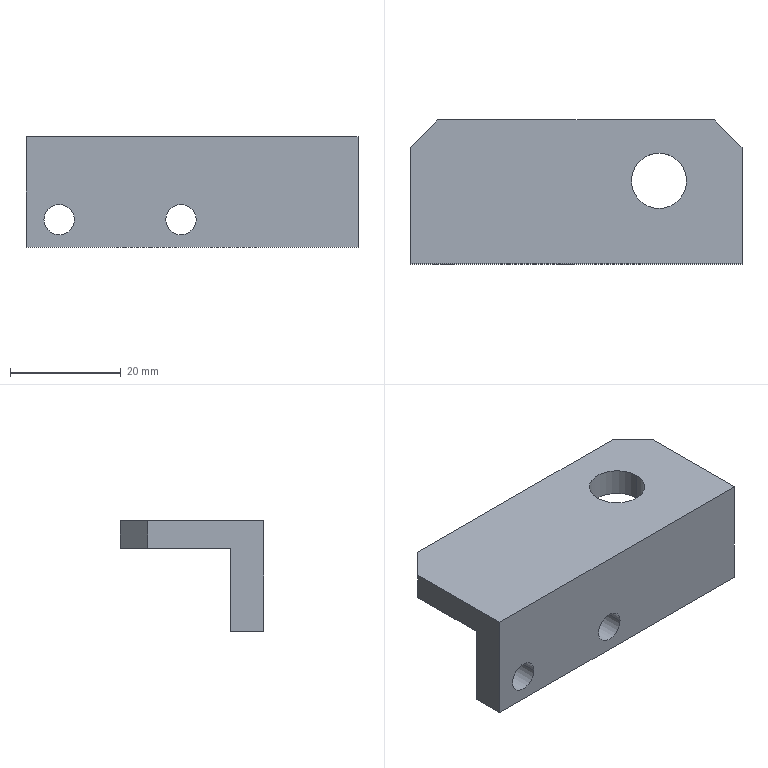Part | STEP file | push slingshot cylinder seat 2 | 1 solid | 16 faces | box 60 x 26 x 20 mm | volume 12397 mm3 | plane 10 | cylinder 6 | commonest cylinder face diameters 5.5 x4 10 x2
STEP:
#1=CARTESIAN_POINT('',(0.,0.,0.));
#2=DIRECTION('',(0.,0.,1.));
#3=DIRECTION('',(1.,0.,0.));
#4=AXIS2_PLACEMENT_3D('',#1,#2,#3);
#5=CARTESIAN_POINT('',(-9.945,-51.173,5.));
#6=VERTEX_POINT('',#5);
#7=CARTESIAN_POINT('',(-9.945,-45.173,5.));
#8=VERTEX_POINT('',#7);
#9=CARTESIAN_POINT('',(-9.945,-55.173,5.));
#10=DIRECTION('',(0.,1.,0.));
#11=VECTOR('',#10,1.);
#12=LINE('',#9,#11);
#13=CARTESIAN_POINT('',(-7.195,-55.173,5.));
#14=DIRECTION('',(0.,1.,0.));
#15=DIRECTION('',(-1.,0.,0.));
#16=AXIS2_PLACEMENT_3D('',#13,#14,#15);
#17=CYLINDRICAL_SURFACE('',#16,2.75);
#18=CARTESIAN_POINT('',(6.283,0.));
#19=DIRECTION('',(0.,1.));
#20=VECTOR('',#19,1.);
#21=LINE('',#18,#20);
#22=(GEOMETRIC_REPRESENTATION_CONTEXT(2)PARAMETRIC_REPRESENTATION_CONTEXT()REPRESENTATION_CONTEXT('',''));
#23=DEFINITIONAL_REPRESENTATION('',(#21),#22);
#24=PCURVE('',#17,#23);
#25=CARTESIAN_POINT('',(-7.195,-55.173,5.));
#26=DIRECTION('',(0.,1.,0.));
#27=DIRECTION('',(-1.,0.,0.));
#28=AXIS2_PLACEMENT_3D('',#25,#26,#27);
#29=CYLINDRICAL_SURFACE('',#28,2.75);
#30=CARTESIAN_POINT('',(0.,0.));
#31=DIRECTION('',(0.,1.));
#32=VECTOR('',#31,1.);
#33=LINE('',#30,#32);
#34=(GEOMETRIC_REPRESENTATION_CONTEXT(2)PARAMETRIC_REPRESENTATION_CONTEXT()REPRESENTATION_CONTEXT('',''));
#35=DEFINITIONAL_REPRESENTATION('',(#33),#34);
#36=PCURVE('',#29,#35);
#37=SURFACE_CURVE('',#12,(#24,#36),.PCURVE_S1.);
#38=EDGE_CURVE('',#6,#8,#37,.T.);
#39=ORIENTED_EDGE('',*,*,#38,.T.);
#40=CARTESIAN_POINT('',(-4.445,-45.173,5.));
#41=VERTEX_POINT('',#40);
#42=CARTESIAN_POINT('',(-7.195,-45.173,5.));
#43=DIRECTION('',(0.,1.,0.));
#44=DIRECTION('',(1.,0.,0.));
#45=AXIS2_PLACEMENT_3D('',#42,#43,#44);
#46=CIRCLE('',#45,2.75);
#47=CARTESIAN_POINT('',(3.142,10.));
#48=DIRECTION('',(1.,0.));
#49=VECTOR('',#48,1.);
#50=LINE('',#47,#49);
#51=(GEOMETRIC_REPRESENTATION_CONTEXT(2)PARAMETRIC_REPRESENTATION_CONTEXT()REPRESENTATION_CONTEXT('',''));
#52=DEFINITIONAL_REPRESENTATION('',(#50),#51);
#53=PCURVE('',#17,#52);
#54=CARTESIAN_POINT('',(-41.653,-45.173,-0.5459));
#55=DIRECTION('',(0.,1.,0.));
#56=DIRECTION('',(-1.,0.,0.));
#57=AXIS2_PLACEMENT_3D('',#54,#55,#56);
#58=PLANE('',#57);
#59=CARTESIAN_POINT('',(-34.458,5.546));
#60=DIRECTION('',(-1.,0.));
#61=AXIS2_PLACEMENT_2D('',#59,#60);
#62=CIRCLE('',#61,2.75);
#63=(GEOMETRIC_REPRESENTATION_CONTEXT(2)PARAMETRIC_REPRESENTATION_CONTEXT()REPRESENTATION_CONTEXT('',''));
#64=DEFINITIONAL_REPRESENTATION('',(#62),#63);
#65=PCURVE('',#58,#64);
#66=SURFACE_CURVE('',#46,(#53,#65),.PCURVE_S1.);
#67=EDGE_CURVE('',#41,#8,#66,.T.);
#68=ORIENTED_EDGE('',*,*,#67,.F.);
#69=CARTESIAN_POINT('',(-4.445,-51.173,5.));
#70=VERTEX_POINT('',#69);
#71=CARTESIAN_POINT('',(-4.445,-55.173,5.));
#72=DIRECTION('',(0.,1.,0.));
#73=VECTOR('',#72,1.);
#74=LINE('',#71,#73);
#75=CARTESIAN_POINT('',(3.142,0.));
#76=DIRECTION('',(0.,1.));
#77=VECTOR('',#76,1.);
#78=LINE('',#75,#77);
#79=(GEOMETRIC_REPRESENTATION_CONTEXT(2)PARAMETRIC_REPRESENTATION_CONTEXT()REPRESENTATION_CONTEXT('',''));
#80=DEFINITIONAL_REPRESENTATION('',(#78),#79);
#81=PCURVE('',#17,#80);
#82=CARTESIAN_POINT('',(3.142,0.));
#83=DIRECTION('',(0.,1.));
#84=VECTOR('',#83,1.);
#85=LINE('',#82,#84);
#86=(GEOMETRIC_REPRESENTATION_CONTEXT(2)PARAMETRIC_REPRESENTATION_CONTEXT()REPRESENTATION_CONTEXT('',''));
#87=DEFINITIONAL_REPRESENTATION('',(#85),#86);
#88=PCURVE('',#29,#87);
#89=SURFACE_CURVE('',#74,(#81,#88),.PCURVE_S1.);
#90=EDGE_CURVE('',#70,#41,#89,.T.);
#91=ORIENTED_EDGE('',*,*,#90,.F.);
#92=CARTESIAN_POINT('',(-7.195,-51.173,5.));
#93=DIRECTION('',(0.,1.,0.));
#94=DIRECTION('',(-1.,0.,0.));
#95=AXIS2_PLACEMENT_3D('',#92,#93,#94);
#96=CIRCLE('',#95,2.75);
#97=CARTESIAN_POINT('',(0.,4.));
#98=DIRECTION('',(1.,0.));
#99=VECTOR('',#98,1.);
#100=LINE('',#97,#99);
#101=(GEOMETRIC_REPRESENTATION_CONTEXT(2)PARAMETRIC_REPRESENTATION_CONTEXT()REPRESENTATION_CONTEXT('',''));
#102=DEFINITIONAL_REPRESENTATION('',(#100),#101);
#103=PCURVE('',#17,#102);
#104=CARTESIAN_POINT('',(-35.195,-51.173,20.));
#105=DIRECTION('',(0.,1.,0.));
#106=DIRECTION('',(-1.,0.,0.));
#107=AXIS2_PLACEMENT_3D('',#104,#105,#106);
#108=PLANE('',#107);
#109=CARTESIAN_POINT('',(-28.,-15.));
#110=DIRECTION('',(1.,0.));
#111=AXIS2_PLACEMENT_2D('',#109,#110);
#112=CIRCLE('',#111,2.75);
#113=(GEOMETRIC_REPRESENTATION_CONTEXT(2)PARAMETRIC_REPRESENTATION_CONTEXT()REPRESENTATION_CONTEXT('',''));
#114=DEFINITIONAL_REPRESENTATION('',(#112),#113);
#115=PCURVE('',#108,#114);
#116=SURFACE_CURVE('',#96,(#103,#115),.PCURVE_S1.);
#117=EDGE_CURVE('',#70,#6,#116,.T.);
#118=ORIENTED_EDGE('',*,*,#117,.T.);
#119=EDGE_LOOP('',(#39,#68,#91,#118));
#120=FACE_BOUND('',#119,.F.);
#121=ADVANCED_FACE('',(#120),#17,.F.);
#122=CARTESIAN_POINT('',(-31.945,-51.173,5.));
#123=VERTEX_POINT('',#122);
#124=CARTESIAN_POINT('',(-31.945,-45.173,5.));
#125=VERTEX_POINT('',#124);
#126=CARTESIAN_POINT('',(-31.945,-55.173,5.));
#127=DIRECTION('',(0.,1.,0.));
#128=VECTOR('',#127,1.);
#129=LINE('',#126,#128);
#130=CARTESIAN_POINT('',(-29.195,-55.173,5.));
#131=DIRECTION('',(0.,1.,0.));
#132=DIRECTION('',(-1.,0.,0.));
#133=AXIS2_PLACEMENT_3D('',#130,#131,#132);
#134=CYLINDRICAL_SURFACE('',#133,2.75);
#135=CARTESIAN_POINT('',(6.283,0.));
#136=DIRECTION('',(0.,1.));
#137=VECTOR('',#136,1.);
#138=LINE('',#135,#137);
#139=(GEOMETRIC_REPRESENTATION_CONTEXT(2)PARAMETRIC_REPRESENTATION_CONTEXT()REPRESENTATION_CONTEXT('',''));
#140=DEFINITIONAL_REPRESENTATION('',(#138),#139);
#141=PCURVE('',#134,#140);
#142=CARTESIAN_POINT('',(-29.195,-55.173,5.));
#143=DIRECTION('',(0.,1.,0.));
#144=DIRECTION('',(-1.,0.,0.));
#145=AXIS2_PLACEMENT_3D('',#142,#143,#144);
#146=CYLINDRICAL_SURFACE('',#145,2.75);
#147=CARTESIAN_POINT('',(0.,0.));
#148=DIRECTION('',(0.,1.));
#149=VECTOR('',#148,1.);
#150=LINE('',#147,#149);
#151=(GEOMETRIC_REPRESENTATION_CONTEXT(2)PARAMETRIC_REPRESENTATION_CONTEXT()REPRESENTATION_CONTEXT('',''));
#152=DEFINITIONAL_REPRESENTATION('',(#150),#151);
#153=PCURVE('',#146,#152);
#154=SURFACE_CURVE('',#129,(#141,#153),.PCURVE_S1.);
#155=EDGE_CURVE('',#123,#125,#154,.T.);
#156=ORIENTED_EDGE('',*,*,#155,.T.);
#157=CARTESIAN_POINT('',(-26.445,-45.173,5.));
#158=VERTEX_POINT('',#157);
#159=CARTESIAN_POINT('',(-29.195,-45.173,5.));
#160=DIRECTION('',(0.,1.,0.));
#161=DIRECTION('',(1.,0.,0.));
#162=AXIS2_PLACEMENT_3D('',#159,#160,#161);
#163=CIRCLE('',#162,2.75);
#164=CARTESIAN_POINT('',(3.142,10.));
#165=DIRECTION('',(1.,0.));
#166=VECTOR('',#165,1.);
#167=LINE('',#164,#166);
#168=(GEOMETRIC_REPRESENTATION_CONTEXT(2)PARAMETRIC_REPRESENTATION_CONTEXT()REPRESENTATION_CONTEXT('',''));
#169=DEFINITIONAL_REPRESENTATION('',(#167),#168);
#170=PCURVE('',#134,#169);
#171=CARTESIAN_POINT('',(-12.458,5.546));
#172=DIRECTION('',(-1.,0.));
#173=AXIS2_PLACEMENT_2D('',#171,#172);
#174=CIRCLE('',#173,2.75);
#175=(GEOMETRIC_REPRESENTATION_CONTEXT(2)PARAMETRIC_REPRESENTATION_CONTEXT()REPRESENTATION_CONTEXT('',''));
#176=DEFINITIONAL_REPRESENTATION('',(#174),#175);
#177=PCURVE('',#58,#176);
#178=SURFACE_CURVE('',#163,(#170,#177),.PCURVE_S1.);
#179=EDGE_CURVE('',#158,#125,#178,.T.);
#180=ORIENTED_EDGE('',*,*,#179,.F.);
#181=CARTESIAN_POINT('',(-26.445,-51.173,5.));
#182=VERTEX_POINT('',#181);
#183=CARTESIAN_POINT('',(-26.445,-55.173,5.));
#184=DIRECTION('',(0.,1.,0.));
#185=VECTOR('',#184,1.);
#186=LINE('',#183,#185);
#187=CARTESIAN_POINT('',(3.142,0.));
#188=DIRECTION('',(0.,1.));
#189=VECTOR('',#188,1.);
#190=LINE('',#187,#189);
#191=(GEOMETRIC_REPRESENTATION_CONTEXT(2)PARAMETRIC_REPRESENTATION_CONTEXT()REPRESENTATION_CONTEXT('',''));
#192=DEFINITIONAL_REPRESENTATION('',(#190),#191);
#193=PCURVE('',#134,#192);
#194=CARTESIAN_POINT('',(3.142,0.));
#195=DIRECTION('',(0.,1.));
#196=VECTOR('',#195,1.);
#197=LINE('',#194,#196);
#198=(GEOMETRIC_REPRESENTATION_CONTEXT(2)PARAMETRIC_REPRESENTATION_CONTEXT()REPRESENTATION_CONTEXT('',''));
#199=DEFINITIONAL_REPRESENTATION('',(#197),#198);
#200=PCURVE('',#146,#199);
#201=SURFACE_CURVE('',#186,(#193,#200),.PCURVE_S1.);
#202=EDGE_CURVE('',#182,#158,#201,.T.);
#203=ORIENTED_EDGE('',*,*,#202,.F.);
#204=CARTESIAN_POINT('',(-29.195,-51.173,5.));
#205=DIRECTION('',(0.,1.,0.));
#206=DIRECTION('',(-1.,0.,0.));
#207=AXIS2_PLACEMENT_3D('',#204,#205,#206);
#208=CIRCLE('',#207,2.75);
#209=CARTESIAN_POINT('',(0.,4.));
#210=DIRECTION('',(1.,0.));
#211=VECTOR('',#210,1.);
#212=LINE('',#209,#211);
#213=(GEOMETRIC_REPRESENTATION_CONTEXT(2)PARAMETRIC_REPRESENTATION_CONTEXT()REPRESENTATION_CONTEXT('',''));
#214=DEFINITIONAL_REPRESENTATION('',(#212),#213);
#215=PCURVE('',#134,#214);
#216=CARTESIAN_POINT('',(-6.,-15.));
#217=DIRECTION('',(1.,0.));
#218=AXIS2_PLACEMENT_2D('',#216,#217);
#219=CIRCLE('',#218,2.75);
#220=(GEOMETRIC_REPRESENTATION_CONTEXT(2)PARAMETRIC_REPRESENTATION_CONTEXT()REPRESENTATION_CONTEXT('',''));
#221=DEFINITIONAL_REPRESENTATION('',(#219),#220);
#222=PCURVE('',#108,#221);
#223=SURFACE_CURVE('',#208,(#215,#222),.PCURVE_S1.);
#224=EDGE_CURVE('',#182,#123,#223,.T.);
#225=ORIENTED_EDGE('',*,*,#224,.T.);
#226=EDGE_LOOP('',(#156,#180,#203,#225));
#227=FACE_BOUND('',#226,.F.);
#228=ADVANCED_FACE('',(#227),#134,.F.);
#229=CARTESIAN_POINT('',(4.805,-36.173,20.));
#230=VERTEX_POINT('',#229);
#231=CARTESIAN_POINT('',(4.805,-36.173,15.));
#232=VERTEX_POINT('',#231);
#233=CARTESIAN_POINT('',(4.805,-36.173,20.));
#234=DIRECTION('',(0.,0.,-1.));
#235=VECTOR('',#234,1.);
#236=LINE('',#233,#235);
#237=CARTESIAN_POINT('',(9.805,-36.173,20.));
#238=DIRECTION('',(0.,0.,-1.));
#239=DIRECTION('',(-1.,0.,0.));
#240=AXIS2_PLACEMENT_3D('',#237,#238,#239);
#241=CYLINDRICAL_SURFACE('',#240,5.);
#242=CARTESIAN_POINT('',(6.283,0.));
#243=DIRECTION('',(0.,1.));
#244=VECTOR('',#243,1.);
#245=LINE('',#242,#244);
#246=(GEOMETRIC_REPRESENTATION_CONTEXT(2)PARAMETRIC_REPRESENTATION_CONTEXT()REPRESENTATION_CONTEXT('',''));
#247=DEFINITIONAL_REPRESENTATION('',(#245),#246);
#248=PCURVE('',#241,#247);
#249=CARTESIAN_POINT('',(9.805,-36.173,20.));
#250=DIRECTION('',(0.,0.,-1.));
#251=DIRECTION('',(-1.,0.,0.));
#252=AXIS2_PLACEMENT_3D('',#249,#250,#251);
#253=CYLINDRICAL_SURFACE('',#252,5.);
#254=CARTESIAN_POINT('',(0.,0.));
#255=DIRECTION('',(0.,1.));
#256=VECTOR('',#255,1.);
#257=LINE('',#254,#256);
#258=(GEOMETRIC_REPRESENTATION_CONTEXT(2)PARAMETRIC_REPRESENTATION_CONTEXT()REPRESENTATION_CONTEXT('',''));
#259=DEFINITIONAL_REPRESENTATION('',(#257),#258);
#260=PCURVE('',#253,#259);
#261=SURFACE_CURVE('',#236,(#248,#260),.PCURVE_S1.);
#262=EDGE_CURVE('',#230,#232,#261,.T.);
#263=ORIENTED_EDGE('',*,*,#262,.T.);
#264=CARTESIAN_POINT('',(14.805,-36.173,15.));
#265=VERTEX_POINT('',#264);
#266=CARTESIAN_POINT('',(9.805,-36.173,15.));
#267=DIRECTION('',(0.,0.,1.));
#268=DIRECTION('',(1.,0.,0.));
#269=AXIS2_PLACEMENT_3D('',#266,#267,#268);
#270=CIRCLE('',#269,5.);
#271=CARTESIAN_POINT('',(9.425,5.));
#272=DIRECTION('',(-1.,0.));
#273=VECTOR('',#272,1.);
#274=LINE('',#271,#273);
#275=(GEOMETRIC_REPRESENTATION_CONTEXT(2)PARAMETRIC_REPRESENTATION_CONTEXT()REPRESENTATION_CONTEXT('',''));
#276=DEFINITIONAL_REPRESENTATION('',(#274),#275);
#277=PCURVE('',#241,#276);
#278=CARTESIAN_POINT('',(-41.653,-45.173,15.));
#279=DIRECTION('',(0.,0.,1.));
#280=DIRECTION('',(1.,0.,0.));
#281=AXIS2_PLACEMENT_3D('',#278,#279,#280);
#282=PLANE('',#281);
#283=CARTESIAN_POINT('',(51.458,9.));
#284=DIRECTION('',(1.,0.));
#285=AXIS2_PLACEMENT_2D('',#283,#284);
#286=CIRCLE('',#285,5.);
#287=(GEOMETRIC_REPRESENTATION_CONTEXT(2)PARAMETRIC_REPRESENTATION_CONTEXT()REPRESENTATION_CONTEXT('',''));
#288=DEFINITIONAL_REPRESENTATION('',(#286),#287);
#289=PCURVE('',#282,#288);
#290=SURFACE_CURVE('',#270,(#277,#289),.PCURVE_S1.);
#291=EDGE_CURVE('',#232,#265,#290,.T.);
#292=ORIENTED_EDGE('',*,*,#291,.T.);
#293=CARTESIAN_POINT('',(14.805,-36.173,20.));
#294=VERTEX_POINT('',#293);
#295=CARTESIAN_POINT('',(14.805,-36.173,20.));
#296=DIRECTION('',(0.,0.,-1.));
#297=VECTOR('',#296,1.);
#298=LINE('',#295,#297);
#299=CARTESIAN_POINT('',(3.142,0.));
#300=DIRECTION('',(0.,1.));
#301=VECTOR('',#300,1.);
#302=LINE('',#299,#301);
#303=(GEOMETRIC_REPRESENTATION_CONTEXT(2)PARAMETRIC_REPRESENTATION_CONTEXT()REPRESENTATION_CONTEXT('',''));
#304=DEFINITIONAL_REPRESENTATION('',(#302),#303);
#305=PCURVE('',#241,#304);
#306=CARTESIAN_POINT('',(3.142,0.));
#307=DIRECTION('',(0.,1.));
#308=VECTOR('',#307,1.);
#309=LINE('',#306,#308);
#310=(GEOMETRIC_REPRESENTATION_CONTEXT(2)PARAMETRIC_REPRESENTATION_CONTEXT()REPRESENTATION_CONTEXT('',''));
#311=DEFINITIONAL_REPRESENTATION('',(#309),#310);
#312=PCURVE('',#253,#311);
#313=SURFACE_CURVE('',#298,(#305,#312),.PCURVE_S1.);
#314=EDGE_CURVE('',#294,#265,#313,.T.);
#315=ORIENTED_EDGE('',*,*,#314,.F.);
#316=CARTESIAN_POINT('',(9.805,-36.173,20.));
#317=DIRECTION('',(0.,0.,1.));
#318=DIRECTION('',(1.,0.,0.));
#319=AXIS2_PLACEMENT_3D('',#316,#317,#318);
#320=CIRCLE('',#319,5.);
#321=CARTESIAN_POINT('',(9.425,0.));
#322=DIRECTION('',(-1.,0.));
#323=VECTOR('',#322,1.);
#324=LINE('',#321,#323);
#325=(GEOMETRIC_REPRESENTATION_CONTEXT(2)PARAMETRIC_REPRESENTATION_CONTEXT()REPRESENTATION_CONTEXT('',''));
#326=DEFINITIONAL_REPRESENTATION('',(#324),#325);
#327=PCURVE('',#241,#326);
#328=CARTESIAN_POINT('',(-35.195,-51.173,20.));
#329=DIRECTION('',(0.,0.,1.));
#330=DIRECTION('',(1.,0.,0.));
#331=AXIS2_PLACEMENT_3D('',#328,#329,#330);
#332=PLANE('',#331);
#333=CARTESIAN_POINT('',(45.,15.));
#334=DIRECTION('',(1.,0.));
#335=AXIS2_PLACEMENT_2D('',#333,#334);
#336=CIRCLE('',#335,5.);
#337=(GEOMETRIC_REPRESENTATION_CONTEXT(2)PARAMETRIC_REPRESENTATION_CONTEXT()REPRESENTATION_CONTEXT('',''));
#338=DEFINITIONAL_REPRESENTATION('',(#336),#337);
#339=PCURVE('',#332,#338);
#340=SURFACE_CURVE('',#320,(#327,#339),.PCURVE_S1.);
#341=EDGE_CURVE('',#230,#294,#340,.T.);
#342=ORIENTED_EDGE('',*,*,#341,.F.);
#343=EDGE_LOOP('',(#263,#292,#315,#342));
#344=FACE_BOUND('',#343,.F.);
#345=ADVANCED_FACE('',(#344),#241,.F.);
#346=CARTESIAN_POINT('',(24.805,-45.173,0.));
#347=VERTEX_POINT('',#346);
#348=CARTESIAN_POINT('',(-35.195,-45.173,0.));
#349=VERTEX_POINT('',#348);
#350=CARTESIAN_POINT('',(-35.195,-45.173,0.));
#351=DIRECTION('',(-1.,0.,0.));
#352=VECTOR('',#351,1.);
#353=LINE('',#350,#352);
#354=CARTESIAN_POINT('',(-35.195,-51.173,0.));
#355=DIRECTION('',(0.,0.,1.));
#356=DIRECTION('',(1.,0.,0.));
#357=AXIS2_PLACEMENT_3D('',#354,#355,#356);
#358=PLANE('',#357);
#359=CARTESIAN_POINT('',(0.,6.));
#360=DIRECTION('',(-1.,0.));
#361=VECTOR('',#360,1.);
#362=LINE('',#359,#361);
#363=(GEOMETRIC_REPRESENTATION_CONTEXT(2)PARAMETRIC_REPRESENTATION_CONTEXT()REPRESENTATION_CONTEXT('',''));
#364=DEFINITIONAL_REPRESENTATION('',(#362),#363);
#365=PCURVE('',#358,#364);
#366=CARTESIAN_POINT('',(-6.458,0.5459));
#367=DIRECTION('',(1.,0.));
#368=VECTOR('',#367,1.);
#369=LINE('',#366,#368);
#370=(GEOMETRIC_REPRESENTATION_CONTEXT(2)PARAMETRIC_REPRESENTATION_CONTEXT()REPRESENTATION_CONTEXT('',''));
#371=DEFINITIONAL_REPRESENTATION('',(#369),#370);
#372=PCURVE('',#58,#371);
#373=SURFACE_CURVE('',#353,(#365,#372),.PCURVE_S1.);
#374=EDGE_CURVE('',#347,#349,#373,.T.);
#375=ORIENTED_EDGE('',*,*,#374,.F.);
#376=CARTESIAN_POINT('',(24.805,-51.173,0.));
#377=VERTEX_POINT('',#376);
#378=CARTESIAN_POINT('',(24.805,-25.173,0.));
#379=DIRECTION('',(0.,1.,0.));
#380=VECTOR('',#379,1.);
#381=LINE('',#378,#380);
#382=CARTESIAN_POINT('',(60.,26.));
#383=DIRECTION('',(0.,1.));
#384=VECTOR('',#383,1.);
#385=LINE('',#382,#384);
#386=(GEOMETRIC_REPRESENTATION_CONTEXT(2)PARAMETRIC_REPRESENTATION_CONTEXT()REPRESENTATION_CONTEXT('',''));
#387=DEFINITIONAL_REPRESENTATION('',(#385),#386);
#388=PCURVE('',#358,#387);
#389=CARTESIAN_POINT('',(24.805,-25.173,20.));
#390=DIRECTION('',(-1.,0.,0.));
#391=DIRECTION('',(0.,-1.,0.));
#392=AXIS2_PLACEMENT_3D('',#389,#390,#391);
#393=PLANE('',#392);
#394=CARTESIAN_POINT('',(0.,-20.));
#395=DIRECTION('',(-1.,0.));
#396=VECTOR('',#395,1.);
#397=LINE('',#394,#396);
#398=(GEOMETRIC_REPRESENTATION_CONTEXT(2)PARAMETRIC_REPRESENTATION_CONTEXT()REPRESENTATION_CONTEXT('',''));
#399=DEFINITIONAL_REPRESENTATION('',(#397),#398);
#400=PCURVE('',#393,#399);
#401=SURFACE_CURVE('',#381,(#388,#400),.PCURVE_S1.);
#402=EDGE_CURVE('',#377,#347,#401,.T.);
#403=ORIENTED_EDGE('',*,*,#402,.F.);
#404=CARTESIAN_POINT('',(-35.195,-51.173,0.));
#405=VERTEX_POINT('',#404);
#406=CARTESIAN_POINT('',(-35.195,-51.173,0.));
#407=DIRECTION('',(1.,0.,0.));
#408=VECTOR('',#407,1.);
#409=LINE('',#406,#408);
#410=CARTESIAN_POINT('',(0.,0.));
#411=DIRECTION('',(1.,0.));
#412=VECTOR('',#411,1.);
#413=LINE('',#410,#412);
#414=(GEOMETRIC_REPRESENTATION_CONTEXT(2)PARAMETRIC_REPRESENTATION_CONTEXT()REPRESENTATION_CONTEXT('',''));
#415=DEFINITIONAL_REPRESENTATION('',(#413),#414);
#416=PCURVE('',#358,#415);
#417=CARTESIAN_POINT('',(0.,-20.));
#418=DIRECTION('',(-1.,0.));
#419=VECTOR('',#418,1.);
#420=LINE('',#417,#419);
#421=(GEOMETRIC_REPRESENTATION_CONTEXT(2)PARAMETRIC_REPRESENTATION_CONTEXT()REPRESENTATION_CONTEXT('',''));
#422=DEFINITIONAL_REPRESENTATION('',(#420),#421);
#423=PCURVE('',#108,#422);
#424=SURFACE_CURVE('',#409,(#416,#423),.PCURVE_S1.);
#425=EDGE_CURVE('',#405,#377,#424,.T.);
#426=ORIENTED_EDGE('',*,*,#425,.F.);
#427=CARTESIAN_POINT('',(-35.195,-25.173,0.));
#428=DIRECTION('',(0.,-1.,0.));
#429=VECTOR('',#428,1.);
#430=LINE('',#427,#429);
#431=CARTESIAN_POINT('',(0.,26.));
#432=DIRECTION('',(0.,-1.));
#433=VECTOR('',#432,1.);
#434=LINE('',#431,#433);
#435=(GEOMETRIC_REPRESENTATION_CONTEXT(2)PARAMETRIC_REPRESENTATION_CONTEXT()REPRESENTATION_CONTEXT('',''));
#436=DEFINITIONAL_REPRESENTATION('',(#434),#435);
#437=PCURVE('',#358,#436);
#438=CARTESIAN_POINT('',(-35.195,-25.173,20.));
#439=DIRECTION('',(1.,0.,0.));
#440=DIRECTION('',(0.,1.,0.));
#441=AXIS2_PLACEMENT_3D('',#438,#439,#440);
#442=PLANE('',#441);
#443=CARTESIAN_POINT('',(0.,-20.));
#444=DIRECTION('',(-1.,0.));
#445=VECTOR('',#444,1.);
#446=LINE('',#443,#445);
#447=(GEOMETRIC_REPRESENTATION_CONTEXT(2)PARAMETRIC_REPRESENTATION_CONTEXT()REPRESENTATION_CONTEXT('',''));
#448=DEFINITIONAL_REPRESENTATION('',(#446),#447);
#449=PCURVE('',#442,#448);
#450=SURFACE_CURVE('',#430,(#437,#449),.PCURVE_S1.);
#451=EDGE_CURVE('',#349,#405,#450,.T.);
#452=ORIENTED_EDGE('',*,*,#451,.F.);
#453=EDGE_LOOP('',(#375,#403,#426,#452));
#454=FACE_BOUND('',#453,.T.);
#455=ADVANCED_FACE('',(#454),#358,.F.);
#456=CARTESIAN_POINT('',(19.805,-25.173,20.));
#457=VERTEX_POINT('',#456);
#458=CARTESIAN_POINT('',(-30.195,-25.173,20.));
#459=VERTEX_POINT('',#458);
#460=CARTESIAN_POINT('',(-35.195,-25.173,20.));
#461=DIRECTION('',(-1.,0.,0.));
#462=VECTOR('',#461,1.);
#463=LINE('',#460,#462);
#464=CARTESIAN_POINT('',(0.,26.));
#465=DIRECTION('',(-1.,0.));
#466=VECTOR('',#465,1.);
#467=LINE('',#464,#466);
#468=(GEOMETRIC_REPRESENTATION_CONTEXT(2)PARAMETRIC_REPRESENTATION_CONTEXT()REPRESENTATION_CONTEXT('',''));
#469=DEFINITIONAL_REPRESENTATION('',(#467),#468);
#470=PCURVE('',#332,#469);
#471=CARTESIAN_POINT('',(-35.195,-25.173,20.));
#472=DIRECTION('',(0.,-1.,0.));
#473=DIRECTION('',(0.,0.,-1.));
#474=AXIS2_PLACEMENT_3D('',#471,#472,#473);
#475=PLANE('',#474);
#476=CARTESIAN_POINT('',(0.,0.));
#477=DIRECTION('',(0.,-1.));
#478=VECTOR('',#477,1.);
#479=LINE('',#476,#478);
#480=(GEOMETRIC_REPRESENTATION_CONTEXT(2)PARAMETRIC_REPRESENTATION_CONTEXT()REPRESENTATION_CONTEXT('',''));
#481=DEFINITIONAL_REPRESENTATION('',(#479),#480);
#482=PCURVE('',#475,#481);
#483=SURFACE_CURVE('',#463,(#470,#482),.PCURVE_S1.);
#484=EDGE_CURVE('',#457,#459,#483,.T.);
#485=ORIENTED_EDGE('',*,*,#484,.T.);
#486=CARTESIAN_POINT('',(-35.195,-30.173,20.));
#487=VERTEX_POINT('',#486);
#488=CARTESIAN_POINT('',(-45.695,-40.673,20.));
#489=DIRECTION('',(-0.7071,-0.7071,0.));
#490=VECTOR('',#489,1.);
#491=LINE('',#488,#490);
#492=CARTESIAN_POINT('',(-10.5,10.5));
#493=DIRECTION('',(-0.7071,-0.7071));
#494=VECTOR('',#493,1.);
#495=LINE('',#492,#494);
#496=(GEOMETRIC_REPRESENTATION_CONTEXT(2)PARAMETRIC_REPRESENTATION_CONTEXT()REPRESENTATION_CONTEXT('',''));
#497=DEFINITIONAL_REPRESENTATION('',(#495),#496);
#498=PCURVE('',#332,#497);
#499=CARTESIAN_POINT('',(-35.195,-30.173,20.));
#500=DIRECTION('',(0.7071,-0.7071,0.));
#501=DIRECTION('',(0.7071,0.7071,0.));
#502=AXIS2_PLACEMENT_3D('',#499,#500,#501);
#503=PLANE('',#502);
#504=CARTESIAN_POINT('',(-14.849,0.));
#505=DIRECTION('',(-1.,0.));
#506=VECTOR('',#505,1.);
#507=LINE('',#504,#506);
#508=(GEOMETRIC_REPRESENTATION_CONTEXT(2)PARAMETRIC_REPRESENTATION_CONTEXT()REPRESENTATION_CONTEXT('',''));
#509=DEFINITIONAL_REPRESENTATION('',(#507),#508);
#510=PCURVE('',#503,#509);
#511=SURFACE_CURVE('',#491,(#498,#510),.PCURVE_S1.);
#512=EDGE_CURVE('',#459,#487,#511,.T.);
#513=ORIENTED_EDGE('',*,*,#512,.T.);
#514=CARTESIAN_POINT('',(-35.195,-51.173,20.));
#515=VERTEX_POINT('',#514);
#516=CARTESIAN_POINT('',(-35.195,-25.173,20.));
#517=DIRECTION('',(0.,-1.,0.));
#518=VECTOR('',#517,1.);
#519=LINE('',#516,#518);
#520=CARTESIAN_POINT('',(0.,26.));
#521=DIRECTION('',(0.,-1.));
#522=VECTOR('',#521,1.);
#523=LINE('',#520,#522);
#524=(GEOMETRIC_REPRESENTATION_CONTEXT(2)PARAMETRIC_REPRESENTATION_CONTEXT()REPRESENTATION_CONTEXT('',''));
#525=DEFINITIONAL_REPRESENTATION('',(#523),#524);
#526=PCURVE('',#332,#525);
#527=CARTESIAN_POINT('',(0.,0.));
#528=DIRECTION('',(-1.,0.));
#529=VECTOR('',#528,1.);
#530=LINE('',#527,#529);
#531=(GEOMETRIC_REPRESENTATION_CONTEXT(2)PARAMETRIC_REPRESENTATION_CONTEXT()REPRESENTATION_CONTEXT('',''));
#532=DEFINITIONAL_REPRESENTATION('',(#530),#531);
#533=PCURVE('',#442,#532);
#534=SURFACE_CURVE('',#519,(#526,#533),.PCURVE_S1.);
#535=EDGE_CURVE('',#487,#515,#534,.T.);
#536=ORIENTED_EDGE('',*,*,#535,.T.);
#537=CARTESIAN_POINT('',(24.805,-51.173,20.));
#538=VERTEX_POINT('',#537);
#539=CARTESIAN_POINT('',(-35.195,-51.173,20.));
#540=DIRECTION('',(1.,0.,0.));
#541=VECTOR('',#540,1.);
#542=LINE('',#539,#541);
#543=CARTESIAN_POINT('',(0.,0.));
#544=DIRECTION('',(1.,0.));
#545=VECTOR('',#544,1.);
#546=LINE('',#543,#545);
#547=(GEOMETRIC_REPRESENTATION_CONTEXT(2)PARAMETRIC_REPRESENTATION_CONTEXT()REPRESENTATION_CONTEXT('',''));
#548=DEFINITIONAL_REPRESENTATION('',(#546),#547);
#549=PCURVE('',#332,#548);
#550=CARTESIAN_POINT('',(0.,0.));
#551=DIRECTION('',(-1.,0.));
#552=VECTOR('',#551,1.);
#553=LINE('',#550,#552);
#554=(GEOMETRIC_REPRESENTATION_CONTEXT(2)PARAMETRIC_REPRESENTATION_CONTEXT()REPRESENTATION_CONTEXT('',''));
#555=DEFINITIONAL_REPRESENTATION('',(#553),#554);
#556=PCURVE('',#108,#555);
#557=SURFACE_CURVE('',#542,(#549,#556),.PCURVE_S1.);
#558=EDGE_CURVE('',#515,#538,#557,.T.);
#559=ORIENTED_EDGE('',*,*,#558,.T.);
#560=CARTESIAN_POINT('',(24.805,-30.173,20.));
#561=VERTEX_POINT('',#560);
#562=CARTESIAN_POINT('',(24.805,-25.173,20.));
#563=DIRECTION('',(0.,1.,0.));
#564=VECTOR('',#563,1.);
#565=LINE('',#562,#564);
#566=CARTESIAN_POINT('',(60.,26.));
#567=DIRECTION('',(0.,1.));
#568=VECTOR('',#567,1.);
#569=LINE('',#566,#568);
#570=(GEOMETRIC_REPRESENTATION_CONTEXT(2)PARAMETRIC_REPRESENTATION_CONTEXT()REPRESENTATION_CONTEXT('',''));
#571=DEFINITIONAL_REPRESENTATION('',(#569),#570);
#572=PCURVE('',#332,#571);
#573=CARTESIAN_POINT('',(0.,0.));
#574=DIRECTION('',(-1.,0.));
#575=VECTOR('',#574,1.);
#576=LINE('',#573,#575);
#577=(GEOMETRIC_REPRESENTATION_CONTEXT(2)PARAMETRIC_REPRESENTATION_CONTEXT()REPRESENTATION_CONTEXT('',''));
#578=DEFINITIONAL_REPRESENTATION('',(#576),#577);
#579=PCURVE('',#393,#578);
#580=SURFACE_CURVE('',#565,(#572,#579),.PCURVE_S1.);
#581=EDGE_CURVE('',#538,#561,#580,.T.);
#582=ORIENTED_EDGE('',*,*,#581,.T.);
#583=CARTESIAN_POINT('',(5.305,-10.673,20.));
#584=DIRECTION('',(-0.7071,0.7071,0.));
#585=VECTOR('',#584,1.);
#586=LINE('',#583,#585);
#587=CARTESIAN_POINT('',(40.5,40.5));
#588=DIRECTION('',(-0.7071,0.7071));
#589=VECTOR('',#588,1.);
#590=LINE('',#587,#589);
#591=(GEOMETRIC_REPRESENTATION_CONTEXT(2)PARAMETRIC_REPRESENTATION_CONTEXT()REPRESENTATION_CONTEXT('',''));
#592=DEFINITIONAL_REPRESENTATION('',(#590),#591);
#593=PCURVE('',#332,#592);
#594=CARTESIAN_POINT('',(19.805,-25.173,20.));
#595=DIRECTION('',(-0.7071,-0.7071,0.));
#596=DIRECTION('',(0.7071,-0.7071,0.));
#597=AXIS2_PLACEMENT_3D('',#594,#595,#596);
#598=PLANE('',#597);
#599=CARTESIAN_POINT('',(-20.506,0.));
#600=DIRECTION('',(-1.,0.));
#601=VECTOR('',#600,1.);
#602=LINE('',#599,#601);
#603=(GEOMETRIC_REPRESENTATION_CONTEXT(2)PARAMETRIC_REPRESENTATION_CONTEXT()REPRESENTATION_CONTEXT('',''));
#604=DEFINITIONAL_REPRESENTATION('',(#602),#603);
#605=PCURVE('',#598,#604);
#606=SURFACE_CURVE('',#586,(#593,#605),.PCURVE_S1.);
#607=EDGE_CURVE('',#561,#457,#606,.T.);
#608=ORIENTED_EDGE('',*,*,#607,.T.);
#609=EDGE_LOOP('',(#485,#513,#536,#559,#582,#608));
#610=FACE_BOUND('',#609,.T.);
#611=ORIENTED_EDGE('',*,*,#341,.F.);
#612=CARTESIAN_POINT('',(9.805,-36.173,20.));
#613=DIRECTION('',(0.,0.,1.));
#614=DIRECTION('',(1.,0.,0.));
#615=AXIS2_PLACEMENT_3D('',#612,#613,#614);
#616=CIRCLE('',#615,5.);
#617=CARTESIAN_POINT('',(45.,15.));
#618=DIRECTION('',(1.,0.));
#619=AXIS2_PLACEMENT_2D('',#617,#618);
#620=CIRCLE('',#619,5.);
#621=(GEOMETRIC_REPRESENTATION_CONTEXT(2)PARAMETRIC_REPRESENTATION_CONTEXT()REPRESENTATION_CONTEXT('',''));
#622=DEFINITIONAL_REPRESENTATION('',(#620),#621);
#623=PCURVE('',#332,#622);
#624=CARTESIAN_POINT('',(3.142,0.));
#625=DIRECTION('',(-1.,0.));
#626=VECTOR('',#625,1.);
#627=LINE('',#624,#626);
#628=(GEOMETRIC_REPRESENTATION_CONTEXT(2)PARAMETRIC_REPRESENTATION_CONTEXT()REPRESENTATION_CONTEXT('',''));
#629=DEFINITIONAL_REPRESENTATION('',(#627),#628);
#630=PCURVE('',#253,#629);
#631=SURFACE_CURVE('',#616,(#623,#630),.PCURVE_S1.);
#632=EDGE_CURVE('',#294,#230,#631,.T.);
#633=ORIENTED_EDGE('',*,*,#632,.F.);
#634=EDGE_LOOP('',(#611,#633));
#635=FACE_BOUND('',#634,.T.);
#636=ADVANCED_FACE('',(#610,#635),#332,.T.);
#637=ORIENTED_EDGE('',*,*,#535,.F.);
#638=CARTESIAN_POINT('',(-35.195,-30.173,15.));
#639=VERTEX_POINT('',#638);
#640=CARTESIAN_POINT('',(-35.195,-30.173,20.));
#641=DIRECTION('',(0.,0.,-1.));
#642=VECTOR('',#641,1.);
#643=LINE('',#640,#642);
#644=CARTESIAN_POINT('',(-5.,0.));
#645=DIRECTION('',(0.,-1.));
#646=VECTOR('',#645,1.);
#647=LINE('',#644,#646);
#648=(GEOMETRIC_REPRESENTATION_CONTEXT(2)PARAMETRIC_REPRESENTATION_CONTEXT()REPRESENTATION_CONTEXT('',''));
#649=DEFINITIONAL_REPRESENTATION('',(#647),#648);
#650=PCURVE('',#442,#649);
#651=CARTESIAN_POINT('',(0.,0.));
#652=DIRECTION('',(0.,-1.));
#653=VECTOR('',#652,1.);
#654=LINE('',#651,#653);
#655=(GEOMETRIC_REPRESENTATION_CONTEXT(2)PARAMETRIC_REPRESENTATION_CONTEXT()REPRESENTATION_CONTEXT('',''));
#656=DEFINITIONAL_REPRESENTATION('',(#654),#655);
#657=PCURVE('',#503,#656);
#658=SURFACE_CURVE('',#643,(#650,#657),.PCURVE_S1.);
#659=EDGE_CURVE('',#487,#639,#658,.T.);
#660=ORIENTED_EDGE('',*,*,#659,.T.);
#661=CARTESIAN_POINT('',(-35.195,-45.173,15.));
#662=VERTEX_POINT('',#661);
#663=CARTESIAN_POINT('',(-35.195,-25.173,15.));
#664=DIRECTION('',(0.,-1.,0.));
#665=VECTOR('',#664,1.);
#666=LINE('',#663,#665);
#667=CARTESIAN_POINT('',(0.,-5.));
#668=DIRECTION('',(-1.,0.));
#669=VECTOR('',#668,1.);
#670=LINE('',#667,#669);
#671=(GEOMETRIC_REPRESENTATION_CONTEXT(2)PARAMETRIC_REPRESENTATION_CONTEXT()REPRESENTATION_CONTEXT('',''));
#672=DEFINITIONAL_REPRESENTATION('',(#670),#671);
#673=PCURVE('',#442,#672);
#674=CARTESIAN_POINT('',(6.458,20.));
#675=DIRECTION('',(0.,-1.));
#676=VECTOR('',#675,1.);
#677=LINE('',#674,#676);
#678=(GEOMETRIC_REPRESENTATION_CONTEXT(2)PARAMETRIC_REPRESENTATION_CONTEXT()REPRESENTATION_CONTEXT('',''));
#679=DEFINITIONAL_REPRESENTATION('',(#677),#678);
#680=PCURVE('',#282,#679);
#681=SURFACE_CURVE('',#666,(#673,#680),.PCURVE_S1.);
#682=EDGE_CURVE('',#639,#662,#681,.T.);
#683=ORIENTED_EDGE('',*,*,#682,.T.);
#684=CARTESIAN_POINT('',(-35.195,-45.173,20.));
#685=DIRECTION('',(0.,0.,1.));
#686=VECTOR('',#685,1.);
#687=LINE('',#684,#686);
#688=CARTESIAN_POINT('',(-20.,0.));
#689=DIRECTION('',(0.,1.));
#690=VECTOR('',#689,1.);
#691=LINE('',#688,#690);
#692=(GEOMETRIC_REPRESENTATION_CONTEXT(2)PARAMETRIC_REPRESENTATION_CONTEXT()REPRESENTATION_CONTEXT('',''));
#693=DEFINITIONAL_REPRESENTATION('',(#691),#692);
#694=PCURVE('',#442,#693);
#695=CARTESIAN_POINT('',(-6.458,20.546));
#696=DIRECTION('',(0.,1.));
#697=VECTOR('',#696,1.);
#698=LINE('',#695,#697);
#699=(GEOMETRIC_REPRESENTATION_CONTEXT(2)PARAMETRIC_REPRESENTATION_CONTEXT()REPRESENTATION_CONTEXT('',''));
#700=DEFINITIONAL_REPRESENTATION('',(#698),#699);
#701=PCURVE('',#58,#700);
#702=SURFACE_CURVE('',#687,(#694,#701),.PCURVE_S1.);
#703=EDGE_CURVE('',#349,#662,#702,.T.);
#704=ORIENTED_EDGE('',*,*,#703,.F.);
#705=ORIENTED_EDGE('',*,*,#451,.T.);
#706=CARTESIAN_POINT('',(-35.195,-51.173,20.));
#707=DIRECTION('',(0.,0.,-1.));
#708=VECTOR('',#707,1.);
#709=LINE('',#706,#708);
#710=CARTESIAN_POINT('',(-26.,0.));
#711=DIRECTION('',(0.,-1.));
#712=VECTOR('',#711,1.);
#713=LINE('',#710,#712);
#714=(GEOMETRIC_REPRESENTATION_CONTEXT(2)PARAMETRIC_REPRESENTATION_CONTEXT()REPRESENTATION_CONTEXT('',''));
#715=DEFINITIONAL_REPRESENTATION('',(#713),#714);
#716=PCURVE('',#442,#715);
#717=CARTESIAN_POINT('',(0.,0.));
#718=DIRECTION('',(0.,-1.));
#719=VECTOR('',#718,1.);
#720=LINE('',#717,#719);
#721=(GEOMETRIC_REPRESENTATION_CONTEXT(2)PARAMETRIC_REPRESENTATION_CONTEXT()REPRESENTATION_CONTEXT('',''));
#722=DEFINITIONAL_REPRESENTATION('',(#720),#721);
#723=PCURVE('',#108,#722);
#724=SURFACE_CURVE('',#709,(#716,#723),.PCURVE_S1.);
#725=EDGE_CURVE('',#515,#405,#724,.T.);
#726=ORIENTED_EDGE('',*,*,#725,.F.);
#727=EDGE_LOOP('',(#637,#660,#683,#704,#705,#726));
#728=FACE_BOUND('',#727,.T.);
#729=ADVANCED_FACE('',(#728),#442,.F.);
#730=CARTESIAN_POINT('',(-7.195,-51.173,5.));
#731=DIRECTION('',(0.,1.,0.));
#732=DIRECTION('',(-1.,0.,0.));
#733=AXIS2_PLACEMENT_3D('',#730,#731,#732);
#734=CIRCLE('',#733,2.75);
#735=CARTESIAN_POINT('',(-28.,-15.));
#736=DIRECTION('',(1.,0.));
#737=AXIS2_PLACEMENT_2D('',#735,#736);
#738=CIRCLE('',#737,2.75);
#739=(GEOMETRIC_REPRESENTATION_CONTEXT(2)PARAMETRIC_REPRESENTATION_CONTEXT()REPRESENTATION_CONTEXT('',''));
#740=DEFINITIONAL_REPRESENTATION('',(#738),#739);
#741=PCURVE('',#108,#740);
#742=CARTESIAN_POINT('',(0.,4.));
#743=DIRECTION('',(1.,0.));
#744=VECTOR('',#743,1.);
#745=LINE('',#742,#744);
#746=(GEOMETRIC_REPRESENTATION_CONTEXT(2)PARAMETRIC_REPRESENTATION_CONTEXT()REPRESENTATION_CONTEXT('',''));
#747=DEFINITIONAL_REPRESENTATION('',(#745),#746);
#748=PCURVE('',#29,#747);
#749=SURFACE_CURVE('',#734,(#741,#748),.PCURVE_S1.);
#750=EDGE_CURVE('',#6,#70,#749,.T.);
#751=ORIENTED_EDGE('',*,*,#750,.T.);
#752=ORIENTED_EDGE('',*,*,#117,.T.);
#753=EDGE_LOOP('',(#751,#752));
#754=FACE_BOUND('',#753,.T.);
#755=CARTESIAN_POINT('',(-29.195,-51.173,5.));
#756=DIRECTION('',(0.,1.,0.));
#757=DIRECTION('',(-1.,0.,0.));
#758=AXIS2_PLACEMENT_3D('',#755,#756,#757);
#759=CIRCLE('',#758,2.75);
#760=CARTESIAN_POINT('',(-6.,-15.));
#761=DIRECTION('',(1.,0.));
#762=AXIS2_PLACEMENT_2D('',#760,#761);
#763=CIRCLE('',#762,2.75);
#764=(GEOMETRIC_REPRESENTATION_CONTEXT(2)PARAMETRIC_REPRESENTATION_CONTEXT()REPRESENTATION_CONTEXT('',''));
#765=DEFINITIONAL_REPRESENTATION('',(#763),#764);
#766=PCURVE('',#108,#765);
#767=CARTESIAN_POINT('',(0.,4.));
#768=DIRECTION('',(1.,0.));
#769=VECTOR('',#768,1.);
#770=LINE('',#767,#769);
#771=(GEOMETRIC_REPRESENTATION_CONTEXT(2)PARAMETRIC_REPRESENTATION_CONTEXT()REPRESENTATION_CONTEXT('',''));
#772=DEFINITIONAL_REPRESENTATION('',(#770),#771);
#773=PCURVE('',#146,#772);
#774=SURFACE_CURVE('',#759,(#766,#773),.PCURVE_S1.);
#775=EDGE_CURVE('',#123,#182,#774,.T.);
#776=ORIENTED_EDGE('',*,*,#775,.T.);
#777=ORIENTED_EDGE('',*,*,#224,.T.);
#778=EDGE_LOOP('',(#776,#777));
#779=FACE_BOUND('',#778,.T.);
#780=ORIENTED_EDGE('',*,*,#425,.T.);
#781=CARTESIAN_POINT('',(24.805,-51.173,20.));
#782=DIRECTION('',(0.,0.,-1.));
#783=VECTOR('',#782,1.);
#784=LINE('',#781,#783);
#785=CARTESIAN_POINT('',(-60.,0.));
#786=DIRECTION('',(0.,-1.));
#787=VECTOR('',#786,1.);
#788=LINE('',#785,#787);
#789=(GEOMETRIC_REPRESENTATION_CONTEXT(2)PARAMETRIC_REPRESENTATION_CONTEXT()REPRESENTATION_CONTEXT('',''));
#790=DEFINITIONAL_REPRESENTATION('',(#788),#789);
#791=PCURVE('',#108,#790);
#792=CARTESIAN_POINT('',(26.,0.));
#793=DIRECTION('',(0.,-1.));
#794=VECTOR('',#793,1.);
#795=LINE('',#792,#794);
#796=(GEOMETRIC_REPRESENTATION_CONTEXT(2)PARAMETRIC_REPRESENTATION_CONTEXT()REPRESENTATION_CONTEXT('',''));
#797=DEFINITIONAL_REPRESENTATION('',(#795),#796);
#798=PCURVE('',#393,#797);
#799=SURFACE_CURVE('',#784,(#791,#798),.PCURVE_S1.);
#800=EDGE_CURVE('',#538,#377,#799,.T.);
#801=ORIENTED_EDGE('',*,*,#800,.F.);
#802=ORIENTED_EDGE('',*,*,#558,.F.);
#803=ORIENTED_EDGE('',*,*,#725,.T.);
#804=EDGE_LOOP('',(#780,#801,#802,#803));
#805=FACE_BOUND('',#804,.T.);
#806=ADVANCED_FACE('',(#754,#779,#805),#108,.F.);
#807=CARTESIAN_POINT('',(24.805,-45.173,15.));
#808=VERTEX_POINT('',#807);
#809=CARTESIAN_POINT('',(24.805,-30.173,15.));
#810=VERTEX_POINT('',#809);
#811=CARTESIAN_POINT('',(24.805,-25.173,15.));
#812=DIRECTION('',(0.,1.,0.));
#813=VECTOR('',#812,1.);
#814=LINE('',#811,#813);
#815=CARTESIAN_POINT('',(0.,-5.));
#816=DIRECTION('',(-1.,0.));
#817=VECTOR('',#816,1.);
#818=LINE('',#815,#817);
#819=(GEOMETRIC_REPRESENTATION_CONTEXT(2)PARAMETRIC_REPRESENTATION_CONTEXT()REPRESENTATION_CONTEXT('',''));
#820=DEFINITIONAL_REPRESENTATION('',(#818),#819);
#821=PCURVE('',#393,#820);
#822=CARTESIAN_POINT('',(66.458,20.));
#823=DIRECTION('',(0.,1.));
#824=VECTOR('',#823,1.);
#825=LINE('',#822,#824);
#826=(GEOMETRIC_REPRESENTATION_CONTEXT(2)PARAMETRIC_REPRESENTATION_CONTEXT()REPRESENTATION_CONTEXT('',''));
#827=DEFINITIONAL_REPRESENTATION('',(#825),#826);
#828=PCURVE('',#282,#827);
#829=SURFACE_CURVE('',#814,(#821,#828),.PCURVE_S1.);
#830=EDGE_CURVE('',#808,#810,#829,.T.);
#831=ORIENTED_EDGE('',*,*,#830,.T.);
#832=CARTESIAN_POINT('',(24.805,-30.173,20.));
#833=DIRECTION('',(0.,0.,1.));
#834=VECTOR('',#833,1.);
#835=LINE('',#832,#834);
#836=CARTESIAN_POINT('',(5.,0.));
#837=DIRECTION('',(0.,1.));
#838=VECTOR('',#837,1.);
#839=LINE('',#836,#838);
#840=(GEOMETRIC_REPRESENTATION_CONTEXT(2)PARAMETRIC_REPRESENTATION_CONTEXT()REPRESENTATION_CONTEXT('',''));
#841=DEFINITIONAL_REPRESENTATION('',(#839),#840);
#842=PCURVE('',#393,#841);
#843=CARTESIAN_POINT('',(7.071,0.));
#844=DIRECTION('',(0.,1.));
#845=VECTOR('',#844,1.);
#846=LINE('',#843,#845);
#847=(GEOMETRIC_REPRESENTATION_CONTEXT(2)PARAMETRIC_REPRESENTATION_CONTEXT()REPRESENTATION_CONTEXT('',''));
#848=DEFINITIONAL_REPRESENTATION('',(#846),#847);
#849=PCURVE('',#598,#848);
#850=SURFACE_CURVE('',#835,(#842,#849),.PCURVE_S1.);
#851=EDGE_CURVE('',#810,#561,#850,.T.);
#852=ORIENTED_EDGE('',*,*,#851,.T.);
#853=ORIENTED_EDGE('',*,*,#581,.F.);
#854=ORIENTED_EDGE('',*,*,#800,.T.);
#855=ORIENTED_EDGE('',*,*,#402,.T.);
#856=CARTESIAN_POINT('',(24.805,-45.173,20.));
#857=DIRECTION('',(0.,0.,-1.));
#858=VECTOR('',#857,1.);
#859=LINE('',#856,#858);
#860=CARTESIAN_POINT('',(20.,0.));
#861=DIRECTION('',(0.,-1.));
#862=VECTOR('',#861,1.);
#863=LINE('',#860,#862);
#864=(GEOMETRIC_REPRESENTATION_CONTEXT(2)PARAMETRIC_REPRESENTATION_CONTEXT()REPRESENTATION_CONTEXT('',''));
#865=DEFINITIONAL_REPRESENTATION('',(#863),#864);
#866=PCURVE('',#393,#865);
#867=CARTESIAN_POINT('',(-66.458,20.546));
#868=DIRECTION('',(0.,-1.));
#869=VECTOR('',#868,1.);
#870=LINE('',#867,#869);
#871=(GEOMETRIC_REPRESENTATION_CONTEXT(2)PARAMETRIC_REPRESENTATION_CONTEXT()REPRESENTATION_CONTEXT('',''));
#872=DEFINITIONAL_REPRESENTATION('',(#870),#871);
#873=PCURVE('',#58,#872);
#874=SURFACE_CURVE('',#859,(#866,#873),.PCURVE_S1.);
#875=EDGE_CURVE('',#808,#347,#874,.T.);
#876=ORIENTED_EDGE('',*,*,#875,.F.);
#877=EDGE_LOOP('',(#831,#852,#853,#854,#855,#876));
#878=FACE_BOUND('',#877,.T.);
#879=ADVANCED_FACE('',(#878),#393,.F.);
#880=CARTESIAN_POINT('',(-30.195,-25.173,15.));
#881=VERTEX_POINT('',#880);
#882=CARTESIAN_POINT('',(19.805,-25.173,15.));
#883=VERTEX_POINT('',#882);
#884=CARTESIAN_POINT('',(-41.653,-25.173,15.));
#885=DIRECTION('',(1.,0.,0.));
#886=VECTOR('',#885,1.);
#887=LINE('',#884,#886);
#888=CARTESIAN_POINT('',(5.,-6.458));
#889=DIRECTION('',(0.,1.));
#890=VECTOR('',#889,1.);
#891=LINE('',#888,#890);
#892=(GEOMETRIC_REPRESENTATION_CONTEXT(2)PARAMETRIC_REPRESENTATION_CONTEXT()REPRESENTATION_CONTEXT('',''));
#893=DEFINITIONAL_REPRESENTATION('',(#891),#892);
#894=PCURVE('',#475,#893);
#895=CARTESIAN_POINT('',(0.,20.));
#896=DIRECTION('',(1.,0.));
#897=VECTOR('',#896,1.);
#898=LINE('',#895,#897);
#899=(GEOMETRIC_REPRESENTATION_CONTEXT(2)PARAMETRIC_REPRESENTATION_CONTEXT()REPRESENTATION_CONTEXT('',''));
#900=DEFINITIONAL_REPRESENTATION('',(#898),#899);
#901=PCURVE('',#282,#900);
#902=SURFACE_CURVE('',#887,(#894,#901),.PCURVE_S1.);
#903=EDGE_CURVE('',#881,#883,#902,.T.);
#904=ORIENTED_EDGE('',*,*,#903,.F.);
#905=CARTESIAN_POINT('',(-30.195,-25.173,20.));
#906=DIRECTION('',(0.,0.,1.));
#907=VECTOR('',#906,1.);
#908=LINE('',#905,#907);
#909=CARTESIAN_POINT('',(0.,5.));
#910=DIRECTION('',(-1.,0.));
#911=VECTOR('',#910,1.);
#912=LINE('',#909,#911);
#913=(GEOMETRIC_REPRESENTATION_CONTEXT(2)PARAMETRIC_REPRESENTATION_CONTEXT()REPRESENTATION_CONTEXT('',''));
#914=DEFINITIONAL_REPRESENTATION('',(#912),#913);
#915=PCURVE('',#475,#914);
#916=CARTESIAN_POINT('',(7.071,0.));
#917=DIRECTION('',(0.,1.));
#918=VECTOR('',#917,1.);
#919=LINE('',#916,#918);
#920=(GEOMETRIC_REPRESENTATION_CONTEXT(2)PARAMETRIC_REPRESENTATION_CONTEXT()REPRESENTATION_CONTEXT('',''));
#921=DEFINITIONAL_REPRESENTATION('',(#919),#920);
#922=PCURVE('',#503,#921);
#923=SURFACE_CURVE('',#908,(#915,#922),.PCURVE_S1.);
#924=EDGE_CURVE('',#881,#459,#923,.T.);
#925=ORIENTED_EDGE('',*,*,#924,.T.);
#926=ORIENTED_EDGE('',*,*,#484,.F.);
#927=CARTESIAN_POINT('',(19.805,-25.173,20.));
#928=DIRECTION('',(0.,0.,-1.));
#929=VECTOR('',#928,1.);
#930=LINE('',#927,#929);
#931=CARTESIAN_POINT('',(0.,55.));
#932=DIRECTION('',(1.,0.));
#933=VECTOR('',#932,1.);
#934=LINE('',#931,#933);
#935=(GEOMETRIC_REPRESENTATION_CONTEXT(2)PARAMETRIC_REPRESENTATION_CONTEXT()REPRESENTATION_CONTEXT('',''));
#936=DEFINITIONAL_REPRESENTATION('',(#934),#935);
#937=PCURVE('',#475,#936);
#938=CARTESIAN_POINT('',(0.,0.));
#939=DIRECTION('',(0.,-1.));
#940=VECTOR('',#939,1.);
#941=LINE('',#938,#940);
#942=(GEOMETRIC_REPRESENTATION_CONTEXT(2)PARAMETRIC_REPRESENTATION_CONTEXT()REPRESENTATION_CONTEXT('',''));
#943=DEFINITIONAL_REPRESENTATION('',(#941),#942);
#944=PCURVE('',#598,#943);
#945=SURFACE_CURVE('',#930,(#937,#944),.PCURVE_S1.);
#946=EDGE_CURVE('',#457,#883,#945,.T.);
#947=ORIENTED_EDGE('',*,*,#946,.T.);
#948=EDGE_LOOP('',(#904,#925,#926,#947));
#949=FACE_BOUND('',#948,.T.);
#950=ADVANCED_FACE('',(#949),#475,.F.);
#951=CARTESIAN_POINT('',(9.805,-36.173,15.));
#952=DIRECTION('',(0.,0.,1.));
#953=DIRECTION('',(1.,0.,0.));
#954=AXIS2_PLACEMENT_3D('',#951,#952,#953);
#955=CIRCLE('',#954,5.);
#956=CARTESIAN_POINT('',(3.142,5.));
#957=DIRECTION('',(-1.,0.));
#958=VECTOR('',#957,1.);
#959=LINE('',#956,#958);
#960=(GEOMETRIC_REPRESENTATION_CONTEXT(2)PARAMETRIC_REPRESENTATION_CONTEXT()REPRESENTATION_CONTEXT('',''));
#961=DEFINITIONAL_REPRESENTATION('',(#959),#960);
#962=PCURVE('',#253,#961);
#963=CARTESIAN_POINT('',(51.458,9.));
#964=DIRECTION('',(1.,0.));
#965=AXIS2_PLACEMENT_2D('',#963,#964);
#966=CIRCLE('',#965,5.);
#967=(GEOMETRIC_REPRESENTATION_CONTEXT(2)PARAMETRIC_REPRESENTATION_CONTEXT()REPRESENTATION_CONTEXT('',''));
#968=DEFINITIONAL_REPRESENTATION('',(#966),#967);
#969=PCURVE('',#282,#968);
#970=SURFACE_CURVE('',#955,(#962,#969),.PCURVE_S1.);
#971=EDGE_CURVE('',#265,#232,#970,.T.);
#972=ORIENTED_EDGE('',*,*,#971,.T.);
#973=ORIENTED_EDGE('',*,*,#262,.F.);
#974=ORIENTED_EDGE('',*,*,#632,.F.);
#975=ORIENTED_EDGE('',*,*,#314,.T.);
#976=EDGE_LOOP('',(#972,#973,#974,#975));
#977=FACE_BOUND('',#976,.F.);
#978=ADVANCED_FACE('',(#977),#253,.F.);
#979=CARTESIAN_POINT('',(-7.195,-45.173,5.));
#980=DIRECTION('',(0.,1.,0.));
#981=DIRECTION('',(1.,0.,0.));
#982=AXIS2_PLACEMENT_3D('',#979,#980,#981);
#983=CIRCLE('',#982,2.75);
#984=CARTESIAN_POINT('',(-34.458,5.546));
#985=DIRECTION('',(-1.,0.));
#986=AXIS2_PLACEMENT_2D('',#984,#985);
#987=CIRCLE('',#986,2.75);
#988=(GEOMETRIC_REPRESENTATION_CONTEXT(2)PARAMETRIC_REPRESENTATION_CONTEXT()REPRESENTATION_CONTEXT('',''));
#989=DEFINITIONAL_REPRESENTATION('',(#987),#988);
#990=PCURVE('',#58,#989);
#991=CARTESIAN_POINT('',(-3.142,10.));
#992=DIRECTION('',(1.,0.));
#993=VECTOR('',#992,1.);
#994=LINE('',#991,#993);
#995=(GEOMETRIC_REPRESENTATION_CONTEXT(2)PARAMETRIC_REPRESENTATION_CONTEXT()REPRESENTATION_CONTEXT('',''));
#996=DEFINITIONAL_REPRESENTATION('',(#994),#995);
#997=PCURVE('',#29,#996);
#998=SURFACE_CURVE('',#983,(#990,#997),.PCURVE_S1.);
#999=EDGE_CURVE('',#8,#41,#998,.T.);
#1000=ORIENTED_EDGE('',*,*,#999,.F.);
#1001=ORIENTED_EDGE('',*,*,#67,.F.);
#1002=EDGE_LOOP('',(#1000,#1001));
#1003=FACE_BOUND('',#1002,.T.);
#1004=CARTESIAN_POINT('',(-29.195,-45.173,5.));
#1005=DIRECTION('',(0.,1.,0.));
#1006=DIRECTION('',(1.,0.,0.));
#1007=AXIS2_PLACEMENT_3D('',#1004,#1005,#1006);
#1008=CIRCLE('',#1007,2.75);
#1009=CARTESIAN_POINT('',(-12.458,5.546));
#1010=DIRECTION('',(-1.,0.));
#1011=AXIS2_PLACEMENT_2D('',#1009,#1010);
#1012=CIRCLE('',#1011,2.75);
#1013=(GEOMETRIC_REPRESENTATION_CONTEXT(2)PARAMETRIC_REPRESENTATION_CONTEXT()REPRESENTATION_CONTEXT('',''));
#1014=DEFINITIONAL_REPRESENTATION('',(#1012),#1013);
#1015=PCURVE('',#58,#1014);
#1016=CARTESIAN_POINT('',(-3.142,10.));
#1017=DIRECTION('',(1.,0.));
#1018=VECTOR('',#1017,1.);
#1019=LINE('',#1016,#1018);
#1020=(GEOMETRIC_REPRESENTATION_CONTEXT(2)PARAMETRIC_REPRESENTATION_CONTEXT()REPRESENTATION_CONTEXT('',''));
#1021=DEFINITIONAL_REPRESENTATION('',(#1019),#1020);
#1022=PCURVE('',#146,#1021);
#1023=SURFACE_CURVE('',#1008,(#1015,#1022),.PCURVE_S1.);
#1024=EDGE_CURVE('',#125,#158,#1023,.T.);
#1025=ORIENTED_EDGE('',*,*,#1024,.F.);
#1026=ORIENTED_EDGE('',*,*,#179,.F.);
#1027=EDGE_LOOP('',(#1025,#1026));
#1028=FACE_BOUND('',#1027,.T.);
#1029=ORIENTED_EDGE('',*,*,#703,.T.);
#1030=CARTESIAN_POINT('',(-41.653,-45.173,15.));
#1031=DIRECTION('',(1.,0.,0.));
#1032=VECTOR('',#1031,1.);
#1033=LINE('',#1030,#1032);
#1034=CARTESIAN_POINT('',(0.,15.546));
#1035=DIRECTION('',(-1.,0.));
#1036=VECTOR('',#1035,1.);
#1037=LINE('',#1034,#1036);
#1038=(GEOMETRIC_REPRESENTATION_CONTEXT(2)PARAMETRIC_REPRESENTATION_CONTEXT()REPRESENTATION_CONTEXT('',''));
#1039=DEFINITIONAL_REPRESENTATION('',(#1037),#1038);
#1040=PCURVE('',#58,#1039);
#1041=CARTESIAN_POINT('',(0.,0.));
#1042=DIRECTION('',(1.,0.));
#1043=VECTOR('',#1042,1.);
#1044=LINE('',#1041,#1043);
#1045=(GEOMETRIC_REPRESENTATION_CONTEXT(2)PARAMETRIC_REPRESENTATION_CONTEXT()REPRESENTATION_CONTEXT('',''));
#1046=DEFINITIONAL_REPRESENTATION('',(#1044),#1045);
#1047=PCURVE('',#282,#1046);
#1048=SURFACE_CURVE('',#1033,(#1040,#1047),.PCURVE_S1.);
#1049=EDGE_CURVE('',#662,#808,#1048,.T.);
#1050=ORIENTED_EDGE('',*,*,#1049,.T.);
#1051=ORIENTED_EDGE('',*,*,#875,.T.);
#1052=ORIENTED_EDGE('',*,*,#374,.T.);
#1053=EDGE_LOOP('',(#1029,#1050,#1051,#1052));
#1054=FACE_BOUND('',#1053,.T.);
#1055=ADVANCED_FACE('',(#1003,#1028,#1054),#58,.T.);
#1056=ORIENTED_EDGE('',*,*,#291,.T.);
#1057=ORIENTED_EDGE('',*,*,#971,.T.);
#1058=EDGE_LOOP('',(#1056,#1057));
#1059=FACE_BOUND('',#1058,.T.);
#1060=ORIENTED_EDGE('',*,*,#682,.F.);
#1061=CARTESIAN_POINT('',(-35.195,-30.173,15.));
#1062=DIRECTION('',(0.7071,0.7071,0.));
#1063=VECTOR('',#1062,1.);
#1064=LINE('',#1061,#1063);
#1065=CARTESIAN_POINT('',(6.458,15.));
#1066=DIRECTION('',(0.7071,0.7071));
#1067=VECTOR('',#1066,1.);
#1068=LINE('',#1065,#1067);
#1069=(GEOMETRIC_REPRESENTATION_CONTEXT(2)PARAMETRIC_REPRESENTATION_CONTEXT()REPRESENTATION_CONTEXT('',''));
#1070=DEFINITIONAL_REPRESENTATION('',(#1068),#1069);
#1071=PCURVE('',#282,#1070);
#1072=CARTESIAN_POINT('',(0.,-5.));
#1073=DIRECTION('',(1.,0.));
#1074=VECTOR('',#1073,1.);
#1075=LINE('',#1072,#1074);
#1076=(GEOMETRIC_REPRESENTATION_CONTEXT(2)PARAMETRIC_REPRESENTATION_CONTEXT()REPRESENTATION_CONTEXT('',''));
#1077=DEFINITIONAL_REPRESENTATION('',(#1075),#1076);
#1078=PCURVE('',#503,#1077);
#1079=SURFACE_CURVE('',#1064,(#1071,#1078),.PCURVE_S1.);
#1080=EDGE_CURVE('',#639,#881,#1079,.T.);
#1081=ORIENTED_EDGE('',*,*,#1080,.T.);
#1082=ORIENTED_EDGE('',*,*,#903,.T.);
#1083=CARTESIAN_POINT('',(19.805,-25.173,15.));
#1084=DIRECTION('',(0.7071,-0.7071,0.));
#1085=VECTOR('',#1084,1.);
#1086=LINE('',#1083,#1085);
#1087=CARTESIAN_POINT('',(61.458,20.));
#1088=DIRECTION('',(0.7071,-0.7071));
#1089=VECTOR('',#1088,1.);
#1090=LINE('',#1087,#1089);
#1091=(GEOMETRIC_REPRESENTATION_CONTEXT(2)PARAMETRIC_REPRESENTATION_CONTEXT()REPRESENTATION_CONTEXT('',''));
#1092=DEFINITIONAL_REPRESENTATION('',(#1090),#1091);
#1093=PCURVE('',#282,#1092);
#1094=CARTESIAN_POINT('',(0.,-5.));
#1095=DIRECTION('',(1.,0.));
#1096=VECTOR('',#1095,1.);
#1097=LINE('',#1094,#1096);
#1098=(GEOMETRIC_REPRESENTATION_CONTEXT(2)PARAMETRIC_REPRESENTATION_CONTEXT()REPRESENTATION_CONTEXT('',''));
#1099=DEFINITIONAL_REPRESENTATION('',(#1097),#1098);
#1100=PCURVE('',#598,#1099);
#1101=SURFACE_CURVE('',#1086,(#1093,#1100),.PCURVE_S1.);
#1102=EDGE_CURVE('',#883,#810,#1101,.T.);
#1103=ORIENTED_EDGE('',*,*,#1102,.T.);
#1104=ORIENTED_EDGE('',*,*,#830,.F.);
#1105=ORIENTED_EDGE('',*,*,#1049,.F.);
#1106=EDGE_LOOP('',(#1060,#1081,#1082,#1103,#1104,#1105));
#1107=FACE_BOUND('',#1106,.T.);
#1108=ADVANCED_FACE('',(#1059,#1107),#282,.F.);
#1109=ORIENTED_EDGE('',*,*,#512,.F.);
#1110=ORIENTED_EDGE('',*,*,#924,.F.);
#1111=ORIENTED_EDGE('',*,*,#1080,.F.);
#1112=ORIENTED_EDGE('',*,*,#659,.F.);
#1113=EDGE_LOOP('',(#1109,#1110,#1111,#1112));
#1114=FACE_BOUND('',#1113,.T.);
#1115=ADVANCED_FACE('',(#1114),#503,.F.);
#1116=ORIENTED_EDGE('',*,*,#607,.F.);
#1117=ORIENTED_EDGE('',*,*,#851,.F.);
#1118=ORIENTED_EDGE('',*,*,#1102,.F.);
#1119=ORIENTED_EDGE('',*,*,#946,.F.);
#1120=EDGE_LOOP('',(#1116,#1117,#1118,#1119));
#1121=FACE_BOUND('',#1120,.T.);
#1122=ADVANCED_FACE('',(#1121),#598,.F.);
#1123=ORIENTED_EDGE('',*,*,#1024,.F.);
#1124=ORIENTED_EDGE('',*,*,#155,.F.);
#1125=ORIENTED_EDGE('',*,*,#775,.T.);
#1126=ORIENTED_EDGE('',*,*,#202,.T.);
#1127=EDGE_LOOP('',(#1123,#1124,#1125,#1126));
#1128=FACE_BOUND('',#1127,.F.);
#1129=ADVANCED_FACE('',(#1128),#146,.F.);
#1130=ORIENTED_EDGE('',*,*,#999,.F.);
#1131=ORIENTED_EDGE('',*,*,#38,.F.);
#1132=ORIENTED_EDGE('',*,*,#750,.T.);
#1133=ORIENTED_EDGE('',*,*,#90,.T.);
#1134=EDGE_LOOP('',(#1130,#1131,#1132,#1133));
#1135=FACE_BOUND('',#1134,.F.);
#1136=ADVANCED_FACE('',(#1135),#29,.F.);
#1137=CLOSED_SHELL('',(#121,#228,#345,#455,#636,#729,#806,#879,#950,#978,#1055,#1108,#1115,#1122,#1129,#1136));
#1138=MANIFOLD_SOLID_BREP('',#1137);
#1139=(LENGTH_UNIT()NAMED_UNIT(*)SI_UNIT(.MILLI.,.METRE.));
#1140=UNCERTAINTY_MEASURE_WITH_UNIT(LENGTH_MEASURE(0.0000001),#1139,'','');
#1141=(NAMED_UNIT(*)PLANE_ANGLE_UNIT()SI_UNIT($,.RADIAN.));
#1142=(NAMED_UNIT(*)SI_UNIT($,.STERADIAN.)SOLID_ANGLE_UNIT());
#1143=(GEOMETRIC_REPRESENTATION_CONTEXT(3)GLOBAL_UNCERTAINTY_ASSIGNED_CONTEXT((#1140))GLOBAL_UNIT_ASSIGNED_CONTEXT((#1139,#1141,#1142))REPRESENTATION_CONTEXT('',''));
#1144=ADVANCED_BREP_SHAPE_REPRESENTATION('',(#4,#1138),#1143);